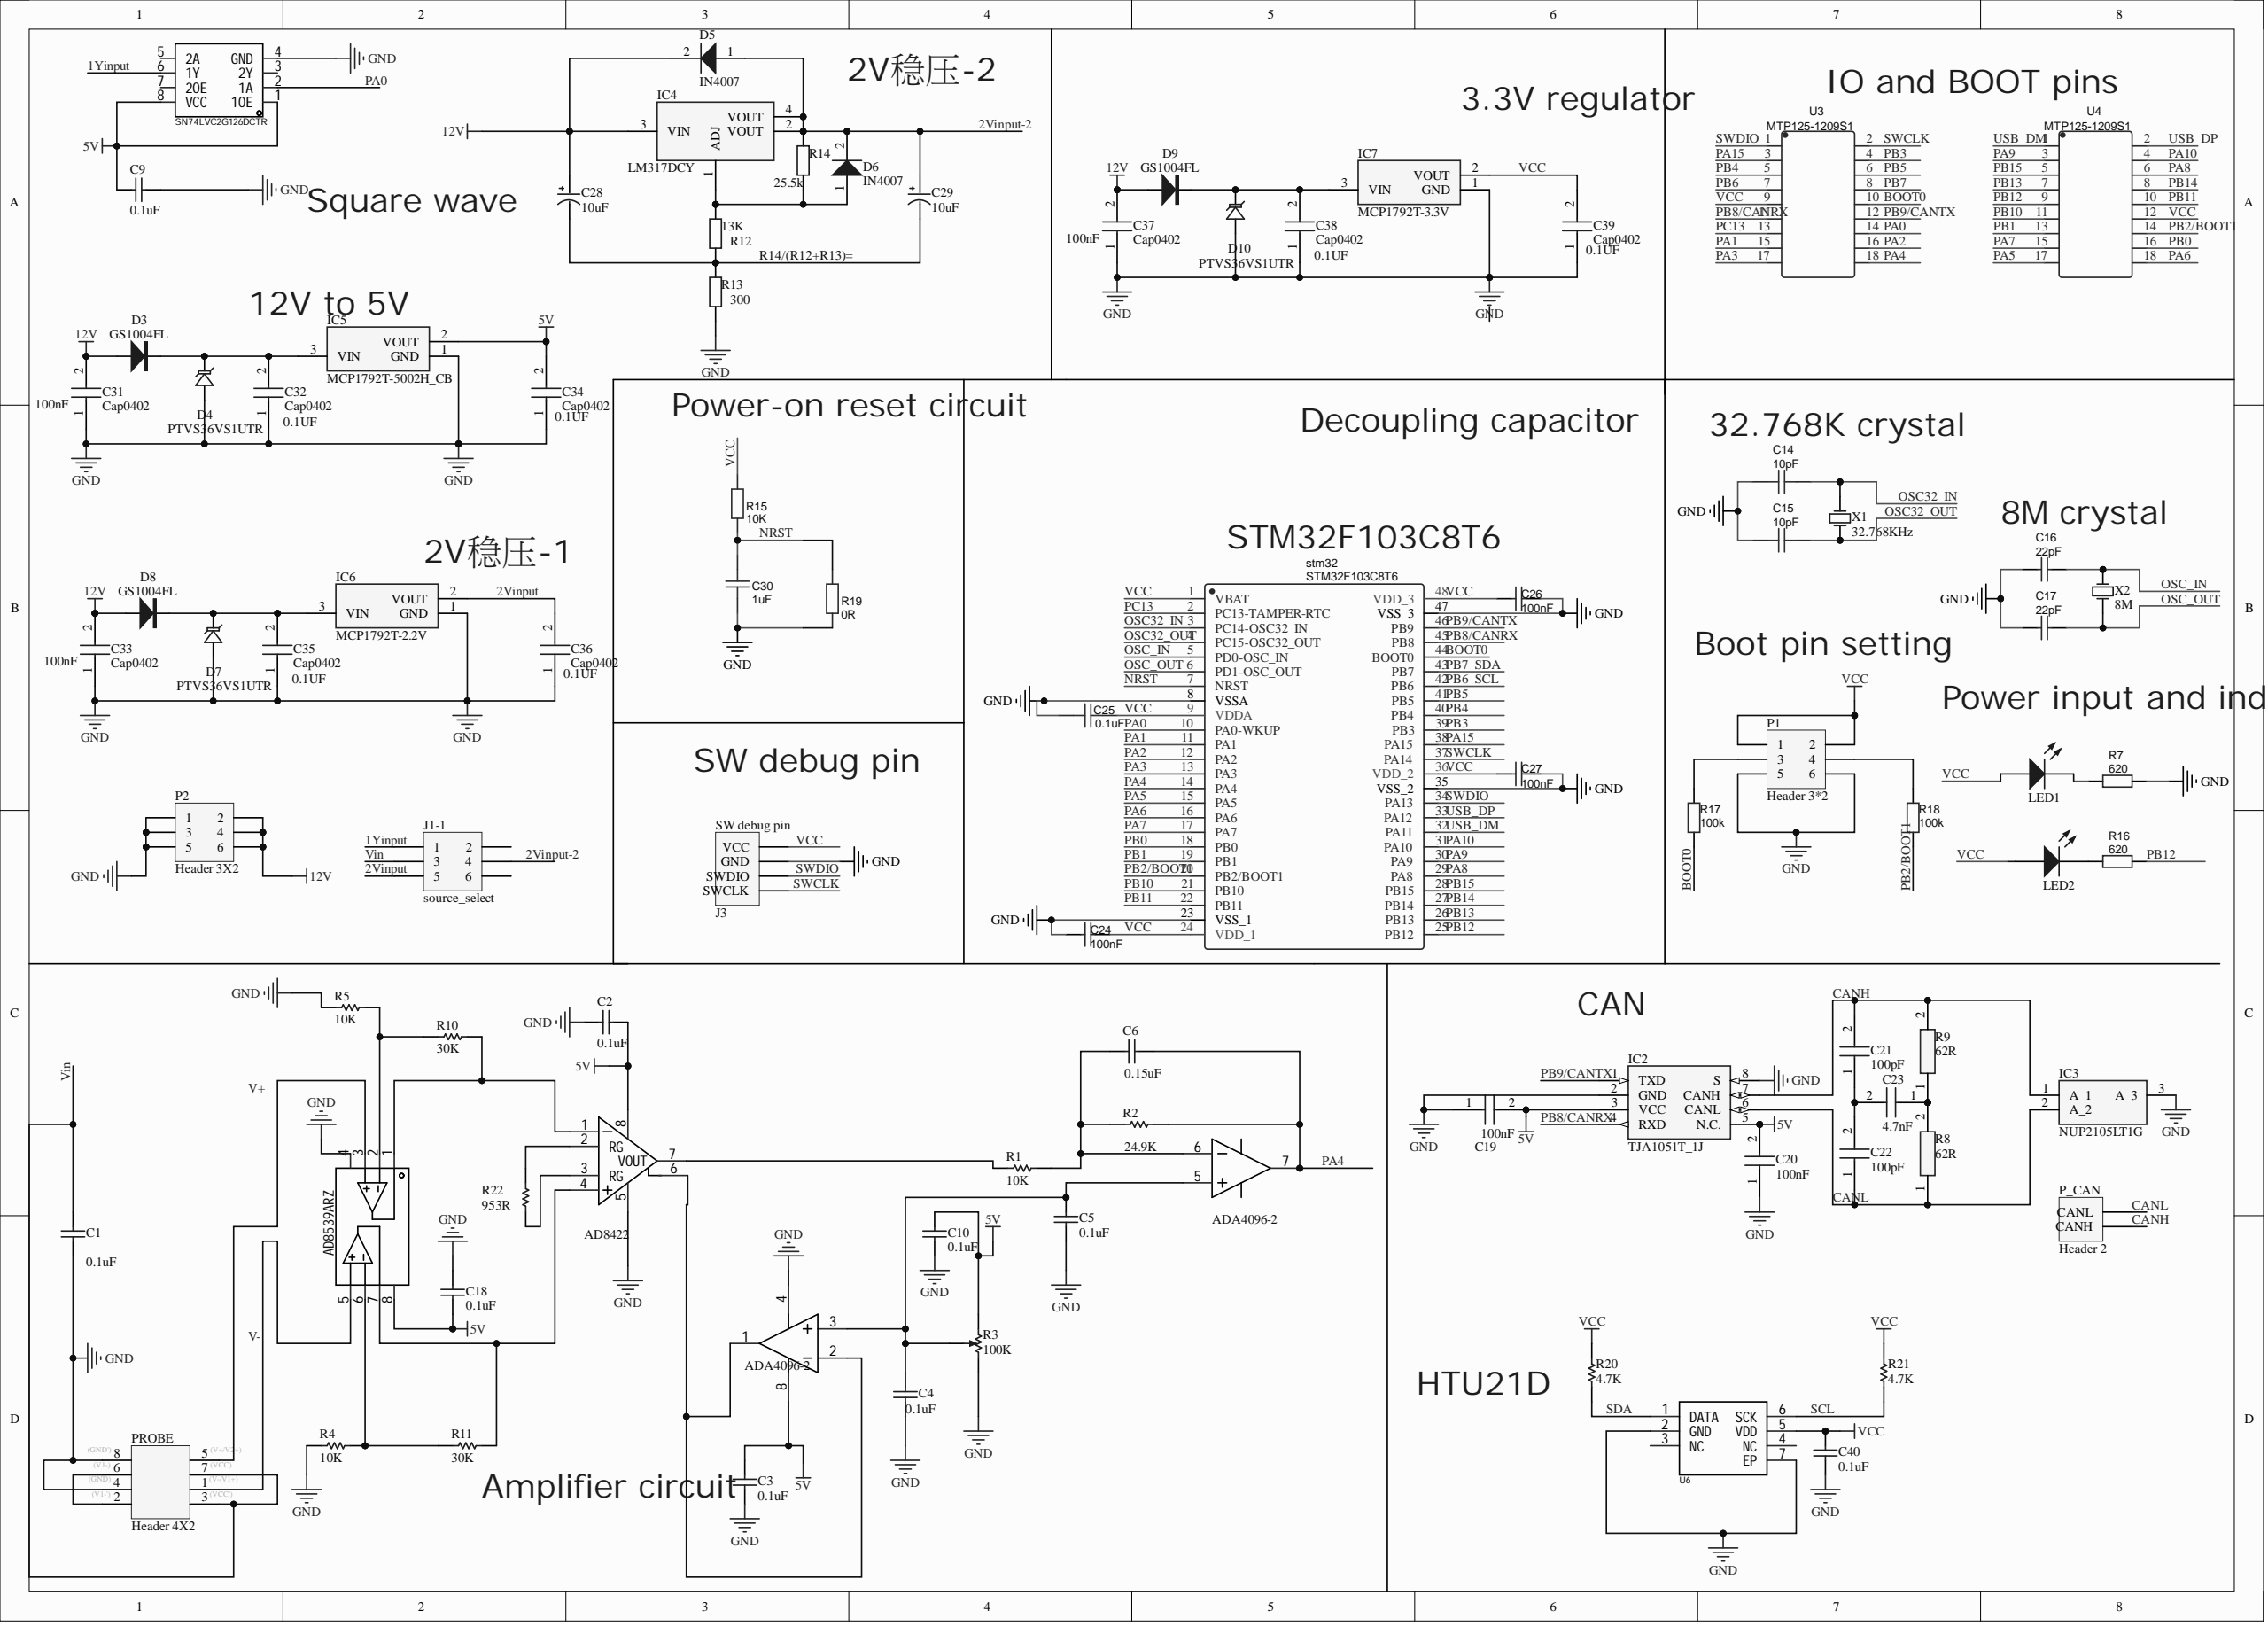Circuit board | Altium Designer | 88 parts | 73 nets
Bill of materials:
Comment,Description,Designator,Footprint,LibRef,Quantity
"Cap","Capacitor","C1, C2, C3, C4, C6, C9, C10, C18, C40","C_C0603_M","Cap","9"
"0.1uF","Capacitor, [NoValue]","C5, C25","C_C0603_M","Cap, 1uF","2"
"10pF","","C14, C15","C_C0603_M","10pF","2"
"22pF","","C16, C17","C_C0603_M","22pF","2"
"100nF","Capacitor","C19, C20","CAPC1005X37N","Cap0402","2"
"100pF","Capacitor","C21, C22","CAPC1005X37N","Cap0402","2"
"4.7nF","Capacitor","C23","CAPC1005X37N","Cap0402","1"
"100nF","","C24, C26, C27","C_C0603_M","100nF","3"
"10uF","","C28, C29","C_R1206","CAP","2"
"1uF","","C30","C_C0603_M","1uF","1"
"Cap0402","Capacitor","C31, C32, C33, C34, C35, C36, C37, C38, C39","C0402","Cap0402","9"
"GS1004FL","Diode","D3, D8, D9","GS1004FL","1N4148","3"
"PTVS36VS1UTR","","D4, D7, D10","PTVS36VS1UTR","TVS","3"
"IN4007","Default Diode","D5, D6","C_DO-214AC","Diode","2"
"TJA1051T_1J","Integrated Circuit","IC2","SOIC-8","TJA1051T_1J","1"
"NUP2105LT1G","Integrated Circuit","IC3","SOT-23A-3","NUP2105LT1G","1"
"LM317DCY","","IC4","SOT223A","LM317DCY","1"
"MCP1792T-5002H_CB","Integrated Circuit","IC5","MCP1792T-220","MCP1792T-3302H_CB","1"
"MCP1792T-2.2V","Integrated Circuit","IC6","MCP1792T-220","MCP1792T-3302H_CB","1"
"MCP1792T-3.3V","Integrated Circuit","IC7","MCP1792T-220","MCP1792T-3302H_CB","1"
"source_select","Header, 3-Pin, Dual row","J1-1","HDR2X3","Header 3X2","1"
"SW debug pin","Connector","J3","HDR4X1_A","Header 4","1"
"LED0","Light-emitting diode","LED1, LED2","LED_0805_Blue","LED0","2"
"Header 3*2","Connector","P1","HDR3X2","Header 3*2","1"
"Header 3X2","Header, 3-Pin, Dual row","P2","HDR2X3","Header 3X2","1"
"Header 2","Header, 2-Pin","P_CAN","HDR1X2","Header 2","1"
"Header 4X2","Header, 4-Pin, Dual row","PROBE","PROBE","Header 4X2","1"
"10K","Resistor, [NoValue]","R1, R4, R5, R15","C_R0603","Res1, 10K","4"
"24.9K","Resistor","R2","C_R0603","Res1","1"
"100K","Square Trimming Potentiometer","R3","VG039N","RPot SM","1"
"620","","R7, R16","C_R0603","620","2"
"62R","Resistor","R8, R9","R0402","Res0402","2"
"30K","Resistor","R10, R11","C_R0603","Res1","2"
"13K","Resistor","R12","C_R0603","SR_110K0603±1%_VISHAY","1"
"300","Resistor","R13","C_R0603","SR_110K0603±1%_VISHAY","1"
"25.5k","Resistor","R14","C_R0603","SR_110K0603±1%_VISHAY","1"
"100k","","R17, R18","C_R0603","620","2"
"0R","","R19","C_R0603","10K","1"
"4.7K","Resistor","R20, R21","C_R0603","Res1","2"
"953R","Resistor","R22","C_R0603","Res1","1"
"SN74LVC2G126DCTR","","SN74LVC2G126DCTR","SN74LVC2G126DCTR1","SN74LVC2G126DCTR","1"
"STM32F103C8T6","","stm32","STM32F103C8T6","STM32F103C8T6","1"
"AD8422ARZ","","U1","AD8422ARZ","AD8422ARZ","1"
"ADA4096-2ARMZ","","U2","ADA4096-2ARMZ","ADA4096-2ARMZ","1"
"MTP125-1209S1","","U3, U4","HEADER2*9","MTP125-1209S1","2"
"AD8539ARZ","","U5","AD8422ARZ","AD8539ARZ","1"
"HTU21D","","U6","htu21d","HTU21D","1"
"32.768KHz","Crystal oscillator","X1","直插晶振-32.768khz","XTAL","1"
"8M","Crystal oscillator","X2","HC-49S_L11.4-W4.8-8HZ","XTAL","1"
Netlist (Protel format):
[
C1
C_C0603_M
Cap



]
[
C2
C_C0603_M
Cap



]
[
C3
C_C0603_M
Cap



]
[
C4
C_C0603_M
Cap



]
[
C5
C_C0603_M
0.1uF



]
[
C6
C_C0603_M
Cap



]
[
C9
C_C0603_M
Cap



]
[
C10
C_C0603_M
Cap



]
[
C14
C_C0603_M
10pF



]
[
C15
C_C0603_M
10pF



]
[
C16
C_C0603_M
22pF



]
[
C17
C_C0603_M
22pF



]
[
C18
C_C0603_M
Cap



]
[
C19
CAPC1005X37N
100nF



]
[
C20
CAPC1005X37N
100nF



]
[
C21
CAPC1005X37N
100pF



]
[
C22
CAPC1005X37N
100pF



]
[
C23
CAPC1005X37N
4.7nF



]
[
C24
C_C0603_M
100nF



]
[
C25
C_C0603_M
0.1uF



]
[
C26
C_C0603_M
100nF



]
[
C27
C_C0603_M
100nF



]
[
C28
C_R1206
10uF



]
[
C29
C_R1206
10uF



]
[
C30
C_C0603_M
1uF



]
[
C31
C0402
Cap0402



]
[
C32
C0402
Cap0402



]
[
C33
C0402
Cap0402



]
[
C34
C0402
Cap0402



]
[
C35
C0402
Cap0402



]
[
C36
C0402
Cap0402



]
[
C37
C0402
Cap0402



]
[
C38
C0402
Cap0402



]
[
C39
C0402
Cap0402



]
[
C40
C_C0603_M
Cap



]
[
D3
GS1004FL
GS1004FL



]
[
D4
PTVS36VS1UTR
PTVS36VS1UTR



]
[
D5
C_DO-214AC
IN4007



]
[
D6
C_DO-214AC
IN4007



]
[
D7
PTVS36VS1UTR
PTVS36VS1UTR



]
[
D8
GS1004FL
GS1004FL



]
[
D9
GS1004FL
GS1004FL



]
[
D10
PTVS36VS1UTR
PTVS36VS1UTR



]
[
IC2
SOIC-8
TJA1051T_1J



]
[
IC3
SOT-23A-3
NUP2105LT1G



]
[
IC4
SOT223A
LM317DCY



]
[
IC5
MCP1792T-220
MCP1792T-5002H_CB



]
[
IC6
MCP1792T-220
MCP1792T-2.2V



]
[
IC7
MCP1792T-220
MCP1792T-3.3V



]
[
J1-1
HDR2X3
source_select



]
[
J3
HDR4X1_A
SW debug pin



]
[
LED1
LED_0805_Blue
LED0



]
[
LED2
LED_0805_Blue
LED0



]
[
P1
HDR3X2
Header 3*2



]
[
P2
HDR2X3
Header 3X2



]
[
P_CAN
HDR1X2
Header 2



]
[
PROBE
PROBE
Header 4X2



]
[
R1
C_R0603
10K



]
[
R2
C_R0603
24.9K



]
[
R3
VG039N
100K



]
[
R4
C_R0603
10K



]
[
R5
C_R0603
10K



]
[
R7
C_R0603
620



]
[
R8
R0402
62R



]
[
R9
R0402
62R



]
[
R10
C_R0603
30K



]
[
R11
C_R0603
30K



]
[
R12
C_R0603
13K



]
[
R13
C_R0603
300



]
[
R14
C_R0603
25.5k



]
[
R15
C_R0603
10K



]
[
R16
C_R0603
620



]
[
R17
C_R0603
100k



]
[
R18
C_R0603
100k



]
[
R19
C_R0603
0R



]
[
R20
C_R0603
4.7K



]
[
R21
C_R0603
4.7K



]
[
R22
C_R0603
953R



]
[
SN74LVC2G126DCTR
SN74LVC2G126DCTR1
SN74LVC2G126DCTR



]
[
stm32
STM32F103C8T6
STM32F103C8T6



]
[
U1
AD8422ARZ
AD8422ARZ



]
[
U2
ADA4096-2ARMZ
ADA4096-2ARMZ



]
[
U3
HEADER2*9
MTP125-1209S1



]
[
U4
HEADER2*9
MTP125-1209S1



]
[
U5
AD8422ARZ
AD8539ARZ



]
[
U6
htu21d
HTU21D



]
[
X1
直插晶振-32.768khz
32.768KHz



]
[
X2
HC-49S_L11.4-W4.8-8HZ
8M



]
(
Vin
C1-2
J1-1-3
PROBE-VCC
PROBE-VCC'
)
(
VCC
C24-2
C25-2
C26-1
C27-1
C39-2
C40-2
IC7-2
J3-4
LED1-1
LED2-1
P1-1
P1-2
R15-2
R20-2
R21-2
stm32-1
stm32-9
stm32-24
stm32-36
stm32-48
U3-9
U4-12
U6-5
)
(
USB_DP
stm32-33
U4-2
)
(
USB_DM
stm32-32
U4-1
)
(
SWDIO
J3-2
stm32-34
U3-1
)
(
SWCLK
J3-1
stm32-37
U3-2
)
(
PC13
stm32-2
U3-13
)
(
PB15
stm32-28
U4-5
)
(
PB14
stm32-27
U4-8
)
(
PB13
stm32-26
U4-7
)
(
PB12
R16-2
stm32-25
U4-9
)
(
PB11
stm32-22
U4-10
)
(
PB10
stm32-21
U4-11
)
(
PB9/CANTX
IC2-1
stm32-46
U3-12
)
(
PB8/CANRX
IC2-4
stm32-45
U3-11
)
(
PB7
R20-1
stm32-43
U3-8
U6-1
)
(
PB6
R21-1
stm32-42
U3-7
U6-6
)
(
PB5
stm32-41
U3-6
)
(
PB4
stm32-40
U3-5
)
(
PB3
stm32-39
U3-4
)
(
PB2/BOOT1
R18-1
stm32-20
U4-14
)
(
PB1
stm32-19
U4-13
)
(
PB0
stm32-18
U4-16
)
(
PA15
stm32-38
U3-3
)
(
PA10
stm32-31
U4-4
)
(
PA9
stm32-30
U4-3
)
(
PA8
stm32-29
U4-6
)
(
PA7
stm32-17
U4-15
)
(
PA6
stm32-16
U4-18
)
(
PA5
stm32-15
U4-17
)
(
PA4
C6-2
R2-2
stm32-14
U2-7
U3-18
)
(
PA3
stm32-13
U3-17
)
(
PA2
stm32-12
U3-16
)
(
PA1
stm32-11
U3-15
)
(
PA0
SN74LVC2G126DCTR-2
stm32-10
U3-14
)
(
OSC_OUT
C17-2
stm32-6
X2-2
)
(
OSC_IN
C16-2
stm32-5
X2-1
)
(
OSC32_OUT
C15-1
stm32-4
X1-2
)
(
OSC32_IN
C14-1
stm32-3
X1-1
)
(
NRST
C30-2
R15-1
R19-2
stm32-7
)
(
NetU1_6
U1-6
U2-1
U2-2
)
(
NetR22_2
R22-2
U1-2
)
(
NetR22_1
R22-1
U1-3
)
(
NetR11_1
R11-1
U1-4
U5-7
)
(
NetR10_1
R10-1
U1-1
U5-1
)
(
NetR5_1
R5-1
R10-2
U5-2
)
(
NetR4_2
R4-2
R11-2
U5-6
)
(
NetR1_1
R1-1
U1-7
)
(
NetPROBE_V-/V1+
PROBE-V-/V1+
U5-5
)
(
NetPROBE_V+/V2+
PROBE-V+/V2+
U5-3
)
(
NetPROBE_V1-
PROBE-V1-
PROBE-V1-'
)
(
NetP1_4
P1-4
R18-2
)
(
NetP1_3
P1-3
R17-2
)
(
NetLED2_2
LED2-2
R16-1
)
(
NetLED1_2
LED1-2
R7-1
)
(
NetD6_1
D6-1
IC4-1
R12-2
R14-1
)
(
NetC38_2
C38-2
D9-2
D10-2
IC7-3
)
(
NetC35_2
C35-2
D7-2
D8-2
IC6-3
)
(
NetC32_2
C32-2
D3-2
D4-2
IC5-3
)
(
NetC28_2
C28-2
C29-2
R12-1
R13-2
)
(
NetC23_1
C23-1
R8-2
R9-1
)
(
NetC21_1
C21-1
C22-2
C23-2
)
(
NetC6_1
C6-1
R1-2
R2-1
U2-6
)
(
NetC4_2
C4-2
C5-2
R3-2
U2-3
U2-5
)
(
GND
C1-1
C2-1
C3-1
C4-1
C5-1
C9-1
C10-1
C14-2
C15-2
C16-1
C17-1
C18-1
C19-1
C20-1
C24-1
C25-1
C26-2
C27-2
C30-1
C31-1
C32-1
C33-1
C34-1
C35-1
C36-1
C37-1
C38-1
C39-1
C40-1
D4-1
D7-1
D10-1
IC2-2
IC2-8
IC3-3
IC5-1
IC6-1
IC7-1
J3-3
P1-5
P1-6
P2-1
P2-3
P2-5
PROBE-GND
PROBE-GND'
R3-1
R4-1
R5-2
R7-2
R13-1
R19-1
SN74LVC2G126DCTR-4
stm32-8
stm32-23
stm32-35
stm32-47
U1-5
U2-4
U5-4
U6-2
U6-7
)
(
CANL
C22-1
IC2-6
IC3-2
P_CAN-2
R8-1
)
(
CANH
C21-2
IC2-7
IC3-1
P_CAN-1
R9-2
)
(
BOOT0
R17-1
stm32-44
U3-10
)
(
12V
C28-1
C31-2
C33-2
C37-2
D3-1
D5-2
D8-1
D9-1
IC4-3
P2-2
P2-4
P2-6
)
(
5V
C2-2
C3-2
C9-2
C10-2
C18-2
C19-2
C20-2
C34-2
IC2-3
IC2-5
IC5-2
R3-3
SN74LVC2G126DCTR-1
SN74LVC2G126DCTR-8
U1-8
U2-8
U5-8
)
(
2Vinput-2
C29-1
D5-1
D6-2
IC4-2
IC4-4
J1-1-4
R14-2
)
(
2Vinput
C36-2
IC6-2
J1-1-5
)
(
1Yinput
J1-1-1
SN74LVC2G126DCTR-6
)